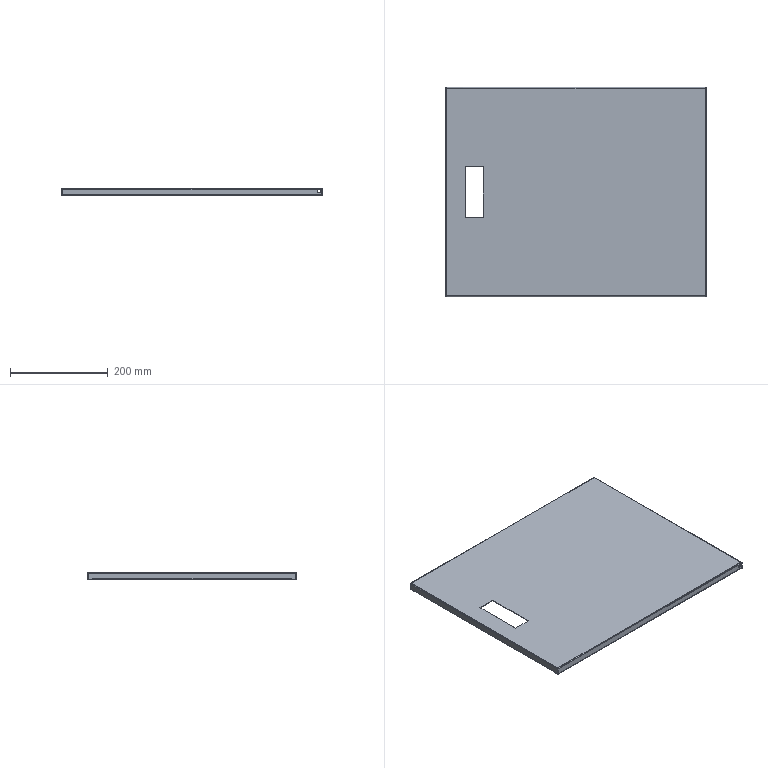Part | STEP file | 1 solid | 102 faces | box 533 x 428 x 15 mm | volume 318433 mm3 | plane 74 | cylinder 20 | spline 8 | commonest cylinder face diameters 1 x8 3.4 x8 7 x4